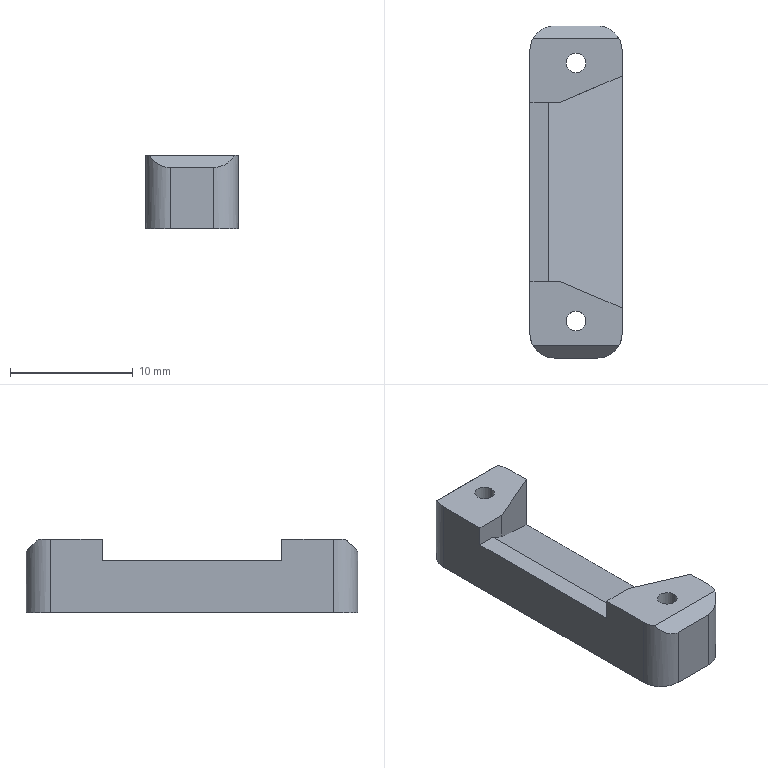NC program | NX | posted with a generic post | part box 7.5 x 27 x 6 mm
Whole program:
N10 G17 G21 G94 G90
(FLOOR_FACING_2 , TOOL : D4-ROUGH)
N12 T01 M6
N14 G54
N16 G17 G0 G90 X0. Y11.08 B0. C0. S4500 M3
N18 G43 Z30.634 H1
N20 Z2.734
N22 G94 G1 Z0.734 F800.
N24 Y5.28
N26 X-4.228
N28 X-3.754 Y4.059
N30 X3.754
N32 X4.228 Y5.28
N34 X0.
N36 Y7.08
N38 X-6.859
N40 X-5.2 Y2.81
N42 Y2.259
N44 X5.2
N46 Y2.81
N48 X6.859 Y7.08
N50 X0.
N52 X-1.
N54 Y11.08
N56 Z2.734
N58 G0 Z30.634
(PLANAR_MILL_4 , TOOL : D4-ROUGH)
N60 X-8.572 Y11.537 S5000
N62 Z2.734
N64 G1 Z0.734
N66 X-7.485 Y8.74
N68 X-5.342 Y3.223
N70 G2 X-5.2 Y2.463 R2.1
N72 G1 Y1.359
N74 Y-1.641
N76 Z2.734
N78 G0 Z30.634
N80 X5.2
N82 Z2.734
N84 G1 Z0.734
N86 Y1.359
N88 Y2.463
N90 G2 X5.342 Y3.223 R2.1
N92 G1 X7.485 Y8.74
N94 X8.572 Y11.537
N96 Z2.734
N98 G0 Z30.634
N100 M5
(FLOOR_FACING_2_COPY , TOOL : D4-FINISH)
N102 T02 M6
N104 G54
N106 G17 G0 G90 X0. Y10.98 B0. C0. S4500 M3
N108 G43 Z30.634 H2
N110 Z2.634
N112 G94 G1 Z0.634 F800.
N114 Y5.18
N116 X-4.279
N118 X-3.882 Y4.159
N120 X3.882
N122 X4.279 Y5.18
N124 X0.
N126 Y6.98
N128 X-6.909
N130 X-5.3 Y2.838
N132 Y2.359
N134 X5.3
N136 Y2.838
N138 X6.909 Y6.98
N140 X0.
N142 X-1.
N144 Y10.98
N146 Z2.634
N148 G0 Z30.634
(PLANAR_MILL_4_COPY , TOOL : D4-FINISH)
N150 X-8.704 Y11.697 S5000
N152 Z2.634
N154 G1 Z0.634
N156 G41 X-8.665 Y11.5 D2
N158 X-7.579 Y8.704
N160 X-5.436 Y3.187
N162 G2 X-5.3 Y2.463 R2.
N164 G1 Y1.359
N166 Y-1.641
N168 G40
N170 X-5.265 Y-1.838
N172 Z2.634
N174 G0 Z30.634
N176 X5.265
N178 Z2.634
N180 G1 Z0.634
N182 G41 X5.3 Y-1.641
N184 Y1.359
N186 Y2.463
N188 G2 X5.436 Y3.187 R2.
N190 G1 X7.579 Y8.704
N192 X8.665 Y11.5
N194 G40
N196 X8.704 Y11.697
N198 Z2.634
N200 G0 Z30.634
N202 M5
(ZLEVEL_PROFILE_STEEP , TOOL : D4R0.3)
N204 T06 M6
N206 G54
N208 G17 G0 G90 X6.252 Y3.561 B0. C0. S4500 M3
N210 G43 Z30.634 H6
N212 Z6.064
N214 G94 G1 Z4.064 F1500.
N216 X7.181 Y5.952
N218 X7.583 Y6.986
N220 Y7.009 Z4.014
N222 X7.13 Y5.845
N224 X7.08 Y5.739 Z3.965
N226 X7.583 Y7.033
N228 Y7.056 Z3.915
N230 X7.03 Y5.632
N232 X6.979 Y5.525 Z3.865
N234 X7.583 Y7.079
N236 Y7.102 Z3.816
N238 X6.929 Y5.419
N240 X6.878 Y5.312 Z3.766
N242 X7.583 Y7.125
N244 Y7.149 Z3.716
N246 X6.828 Y5.206
N248 X6.777 Y5.099 Z3.666
N250 X7.583 Y7.172
N252 Y7.195 Z3.617
N254 X6.727 Y4.992
N256 X6.677 Y4.886 Z3.567
N258 X7.583 Y7.218
N260 Y7.241 Z3.517
N262 X6.626 Y4.779
N264 X6.576 Y4.672 Z3.468
N266 X7.583 Y7.264
N268 Y7.288 Z3.418
N270 X6.546 Y4.619
N272 X6.475 Y4.459 Z3.368
N274 X7.583 Y7.311
N276 Y7.334 Z3.318
N278 X6.425 Y4.353
N280 X6.374 Y4.246 Z3.269
N282 X7.583 Y7.357
N284 Y7.38 Z3.219
N286 X6.324 Y4.139
N288 X6.273 Y4.033 Z3.169
N290 X7.583 Y7.404
N292 Y7.427 Z3.12
N294 X6.223 Y3.926
N296 X6.172 Y3.82 Z3.07
N298 X7.583 Y7.45
N300 Y7.473 Z3.02
N302 X6.122 Y3.713
N304 X6.072 Y3.606 Z2.97
N306 X7.583 Y7.496
N308 Y7.519 Z2.921
N310 X6.021 Y3.5
N312 X5.971 Y3.393 Z2.871
N314 X7.583 Y7.543
N316 Y7.566 Z2.821
N318 X5.92 Y3.287
N320 X5.87 Y3.18 Z2.772
N322 X7.583 Y7.589
N324 Y7.612 Z2.722
N326 X5.82 Y3.073
N328 X5.769 Y2.967 Z2.672
N330 X7.583 Y7.635
N332 Y7.659 Z2.622
N334 X5.719 Y2.86
N336 X5.668 Y2.754 Z2.573
N338 X7.583 Y7.682
N340 Y7.705 Z2.523
N342 X5.618 Y2.647
N344 X5.569 Y2.544 Z2.473
N346 X7.583 Y7.728
N348 Y7.751 Z2.424
N350 X5.517 Y2.434
N352 X5.467 Y2.327 Z2.374
N354 X7.583 Y7.774
N356 Y7.798 Z2.324
N358 X5.44 Y2.281
N360 Y2.304 Z2.274
N362 X7.583 Y7.821
N364 Y7.844 Z2.225
N366 X5.44 Y2.327
N368 Y2.35 Z2.175
N370 X7.583 Y7.867
N372 Y7.89 Z2.125
N374 X5.44 Y2.373
N376 Y2.397 Z2.076
N378 X7.583 Y7.914
N380 Y7.937 Z2.026
N382 X5.44 Y2.42
N384 Y2.443 Z1.976
N386 X7.583 Y7.96
N388 Y7.983 Z1.926
N390 X5.44 Y2.466
N392 Y2.489 Z1.877
N394 X7.583 Y8.006
N396 Y8.029 Z1.827
N398 X5.44 Y2.513
N400 Y2.536 Z1.777
N402 X7.583 Y8.053
N404 Y8.076 Z1.728
N406 X5.44 Y2.559
N408 Y2.582 Z1.678
N410 X7.583 Y8.099
N412 Y8.122 Z1.628
N414 X5.44 Y2.605
N416 Y2.628 Z1.578
N418 X7.583 Y8.145
N420 Y8.169 Z1.529
N422 X5.44 Y2.652
N424 Y2.675 Z1.479
N426 X7.583 Y8.192
N428 Y8.215 Z1.429
N430 X5.44 Y2.698
N432 Y2.721 Z1.38
N434 X7.583 Y8.238
N436 Y8.261 Z1.33
N438 X5.44 Y2.744
N440 Y2.768 Z1.28
N442 X7.583 Y8.284
N444 Y8.308 Z1.23
N446 X5.44 Y2.791
N448 Y2.814 Z1.181
N450 X7.583 Y8.331
N452 Y8.354 Z1.131
N454 X5.44 Y2.837
N456 Y2.86 Z1.081
N458 X7.583 Y8.377
N460 Y8.4 Z1.032
N462 X5.44 Y2.883
N464 Y2.907 Z0.982
N466 X7.583 Y8.424
N468 Y8.447 Z0.932
N470 X5.44 Y2.93
N472 Y2.953 Z0.882
N474 X7.583 Y8.47
N476 Y8.493 Z0.833
N478 X5.44 Y2.976
N480 Y2.999 Z0.783
N482 X7.583 Y8.516
N484 Y8.539 Z0.733
N486 X5.44 Y3.023
N488 Y3.046 Z0.684
N490 X7.583 Y8.563
N492 Y8.585 Z0.634
N494 X5.444 Y3.081
N496 X5.082 Y2.149
N498 X4.3
N500 Z2.634
N502 G0 Z30.634
N504 X-8.396 Y9.081
N506 Z6.064
N508 G1 Z4.064
N510 X-7.583 Y6.986
N512 X-7.181 Y5.952
N514 X-7.13 Y5.845 Z4.014
N516 X-7.583 Y7.009
N518 Y7.033 Z3.965
N520 X-7.08 Y5.739
N522 X-7.03 Y5.632 Z3.915
N524 X-7.583 Y7.056
N526 Y7.079 Z3.865
N528 X-6.979 Y5.525
N530 X-6.929 Y5.419 Z3.816
N532 X-7.583 Y7.102
N534 Y7.125 Z3.766
N536 X-6.878 Y5.312
N538 X-6.828 Y5.206 Z3.716
N540 X-7.583 Y7.149
N542 Y7.172 Z3.666
N544 X-6.777 Y5.099
N546 X-6.727 Y4.992 Z3.617
N548 X-7.583 Y7.195
N550 Y7.218 Z3.567
N552 X-6.677 Y4.886
N554 X-6.626 Y4.779 Z3.517
N556 X-7.583 Y7.241
N558 Y7.264 Z3.468
N560 X-6.576 Y4.672
N562 X-6.546 Y4.619 Z3.418
N564 X-7.583 Y7.288
N566 Y7.311 Z3.368
N568 X-6.475 Y4.459
N570 X-6.425 Y4.353 Z3.318
N572 X-7.583 Y7.334
N574 Y7.357 Z3.269
N576 X-6.374 Y4.246
N578 X-6.324 Y4.139 Z3.219
N580 X-7.583 Y7.38
N582 Y7.404 Z3.169
N584 X-6.273 Y4.033
N586 X-6.223 Y3.926 Z3.12
N588 X-7.583 Y7.427
N590 Y7.45 Z3.07
N592 X-6.172 Y3.82
N594 X-6.122 Y3.713 Z3.02
N596 X-7.583 Y7.473
N598 Y7.496 Z2.97
N600 X-6.072 Y3.606
N602 X-6.021 Y3.5 Z2.921
N604 X-7.583 Y7.519
N606 Y7.543 Z2.871
N608 X-5.971 Y3.393
N610 X-5.92 Y3.287 Z2.821
N612 X-7.583 Y7.566
N614 Y7.589 Z2.772
N616 X-5.87 Y3.18
N618 X-5.82 Y3.073 Z2.722
N620 X-7.583 Y7.612
N622 Y7.635 Z2.672
N624 X-5.769 Y2.967
N626 X-5.719 Y2.86 Z2.622
N628 X-7.583 Y7.659
N630 Y7.682 Z2.573
N632 X-5.668 Y2.754
N634 X-5.618 Y2.647 Z2.523
N636 X-7.583 Y7.705
N638 Y7.728 Z2.473
N640 X-5.569 Y2.544
N642 X-5.517 Y2.434 Z2.424
N644 X-7.583 Y7.751
N646 Y7.774 Z2.374
N648 X-5.467 Y2.327
N650 X-5.444 Y2.292 Z2.324
N652 X-7.583 Y7.798
N654 Y7.821 Z2.274
N656 X-5.44 Y2.304
N658 Y2.327 Z2.225
N660 X-7.583 Y7.844
N662 Y7.867 Z2.175
N664 X-5.44 Y2.35
N666 Y2.373 Z2.125
N668 X-7.583 Y7.89
N670 Y7.914 Z2.076
N672 X-5.44 Y2.397
N674 Y2.42 Z2.026
N676 X-7.583 Y7.937
N678 Y7.96 Z1.976
N680 X-5.44 Y2.443
N682 Y2.466 Z1.926
N684 X-7.583 Y7.983
N686 Y8.006 Z1.877
N688 X-5.44 Y2.489
N690 Y2.513 Z1.827
N692 X-7.583 Y8.029
N694 Y8.053 Z1.777
N696 X-5.44 Y2.536
N698 Y2.559 Z1.728
N700 X-7.583 Y8.076
N702 Y8.099 Z1.678
N704 X-5.44 Y2.582
N706 Y2.605 Z1.628
N708 X-7.583 Y8.122
N710 Y8.145 Z1.578
N712 X-5.44 Y2.628
N714 Y2.652 Z1.529
N716 X-7.583 Y8.169
N718 Y8.192 Z1.479
N720 X-5.44 Y2.675
N722 Y2.698 Z1.429
N724 X-7.583 Y8.215
N726 Y8.238 Z1.38
N728 X-5.44 Y2.721
N730 Y2.744 Z1.33
N732 X-7.583 Y8.261
N734 Y8.284 Z1.28
N736 X-5.44 Y2.768
N738 Y2.791 Z1.23
N740 X-7.583 Y8.308
N742 Y8.331 Z1.181
N744 X-5.44 Y2.814
N746 Y2.837 Z1.131
N748 X-7.583 Y8.354
N750 Y8.377 Z1.081
N752 X-5.44 Y2.86
N754 Y2.883 Z1.032
N756 X-7.583 Y8.4
N758 Y8.424 Z0.982
N760 X-5.44 Y2.907
N762 Y2.93 Z0.932
N764 X-7.583 Y8.447
N766 Y8.47 Z0.882
N768 X-5.44 Y2.953
N770 Y2.976 Z0.833
N772 X-7.583 Y8.493
N774 Y8.516 Z0.783
N776 X-5.44 Y2.999
N778 Y3.023 Z0.733
N780 X-7.583 Y8.539
N782 Y8.563 Z0.684
N784 X-5.44 Y3.046
N786 Y3.069 Z0.634
N788 X-7.583 Y8.585
N790 X-8.396 Y10.679
N792 Z2.634
N794 G0 Z30.634
N796 M5
N798 M2